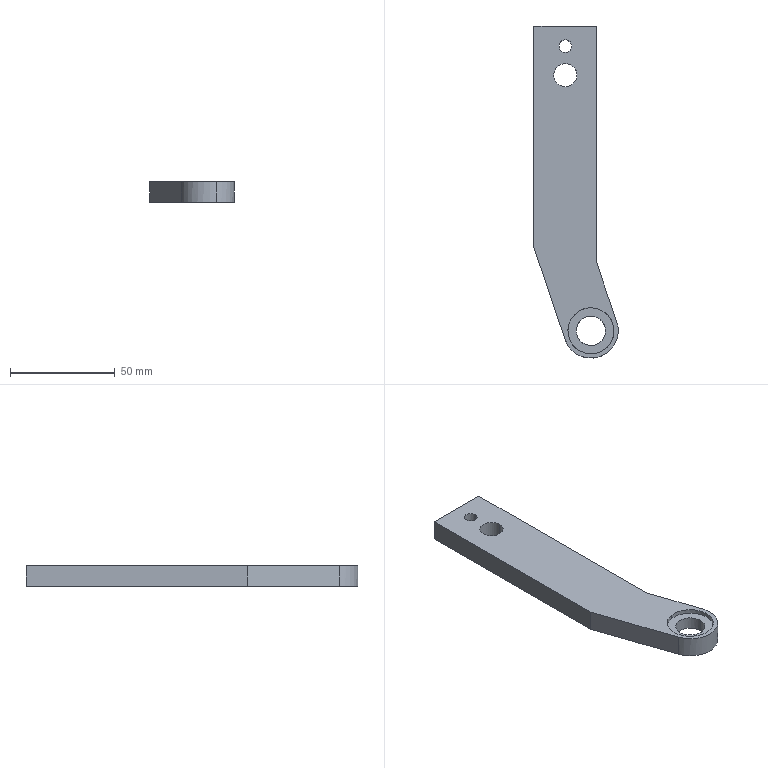Part | SolidWorks | features HoleWzd 2, BaseBody 1, Chamfer 1 | 1 solid | 23 faces | box 40.191 x 158.27 x 10 mm | volume 41618 mm3 | cylinder 12 | plane 9 | cone 2 | commonest cylinder face diameters 22 x4 6 x2 11 x2 14 x2 26 x2
STEP:
#1=CARTESIAN_POINT('',(409.071,348.177,19.477));
#2=VERTEX_POINT('',#1);
#3=CARTESIAN_POINT('',(403.071,348.177,19.477));
#4=VERTEX_POINT('',#3);
#5=CARTESIAN_POINT('',(406.071,348.177,19.477));
#6=DIRECTION('',(0.,0.,-1.));
#7=DIRECTION('',(-1.,0.,0.));
#8=AXIS2_PLACEMENT_3D('',#5,#6,#7);
#9=CIRCLE('',#8,3.);
#10=EDGE_CURVE('',#2,#4,#9,.T.);
#11=ORIENTED_EDGE('',*,*,#10,.F.);
#12=CARTESIAN_POINT('',(410.071,348.177,18.477));
#13=VERTEX_POINT('',#12);
#14=CARTESIAN_POINT('',(409.071,348.177,19.477));
#15=DIRECTION('',(0.7071,0.,-0.7071));
#16=VECTOR('',#15,1000.);
#17=LINE('',#14,#16);
#18=EDGE_CURVE('',#2,#13,#17,.T.);
#19=ORIENTED_EDGE('',*,*,#18,.T.);
#20=CARTESIAN_POINT('',(402.071,348.177,18.477));
#21=VERTEX_POINT('',#20);
#22=CARTESIAN_POINT('',(406.071,348.177,18.477));
#23=DIRECTION('',(0.,0.,1.));
#24=DIRECTION('',(-1.,0.,0.));
#25=AXIS2_PLACEMENT_3D('',#22,#23,#24);
#26=CIRCLE('',#25,4.);
#27=EDGE_CURVE('',#21,#13,#26,.T.);
#28=ORIENTED_EDGE('',*,*,#27,.F.);
#29=CARTESIAN_POINT('',(403.071,348.177,19.477));
#30=DIRECTION('',(-0.7071,0.,-0.7071));
#31=VECTOR('',#30,1000.);
#32=LINE('',#29,#31);
#33=EDGE_CURVE('',#4,#21,#32,.T.);
#34=ORIENTED_EDGE('',*,*,#33,.F.);
#35=EDGE_LOOP('',(#11,#19,#28,#34));
#36=FACE_OUTER_BOUND('',#35,.T.);
#37=CARTESIAN_POINT('',(406.071,348.177,19.477));
#38=DIRECTION('',(0.,0.,-1.));
#39=DIRECTION('',(-1.,0.,0.));
#40=AXIS2_PLACEMENT_3D('',#37,#38,#39);
#41=CONICAL_SURFACE('',#40,3.,0.7854);
#42=ADVANCED_FACE('',(#36),#41,.F.);
#43=CARTESIAN_POINT('',(411.563,334.317,18.477));
#44=VERTEX_POINT('',#43);
#45=CARTESIAN_POINT('',(400.563,334.317,18.477));
#46=VERTEX_POINT('',#45);
#47=CARTESIAN_POINT('',(411.563,334.317,18.477));
#48=CARTESIAN_POINT('',(411.563,323.317,18.477));
#49=CARTESIAN_POINT('',(400.563,323.317,18.477));
#50=CARTESIAN_POINT('',(400.563,334.317,18.477));
#51=(BOUNDED_CURVE()B_SPLINE_CURVE(3,(#47,#48,#49,#50),.UNSPECIFIED.,.F.,.F.)B_SPLINE_CURVE_WITH_KNOTS((4,4),(5.82,8.961),.UNSPECIFIED.)CURVE()GEOMETRIC_REPRESENTATION_ITEM()RATIONAL_B_SPLINE_CURVE((1.,0.3333,0.3333,1.))REPRESENTATION_ITEM(''));
#52=EDGE_CURVE('',#44,#46,#51,.T.);
#53=ORIENTED_EDGE('',*,*,#52,.T.);
#54=CARTESIAN_POINT('',(400.565,334.315,28.477));
#55=VERTEX_POINT('',#54);
#56=CARTESIAN_POINT('',(400.565,334.315,28.48));
#57=DIRECTION('',(0.0002857,-0.0001428,1.));
#58=VECTOR('',#57,1000.);
#59=LINE('',#56,#58);
#60=EDGE_CURVE('',#46,#55,#59,.T.);
#61=ORIENTED_EDGE('',*,*,#60,.T.);
#62=CARTESIAN_POINT('',(411.565,334.315,28.477));
#63=VERTEX_POINT('',#62);
#64=CARTESIAN_POINT('',(411.565,334.315,28.477));
#65=CARTESIAN_POINT('',(411.565,323.315,28.477));
#66=CARTESIAN_POINT('',(400.565,323.315,28.477));
#67=CARTESIAN_POINT('',(400.565,334.315,28.477));
#68=(BOUNDED_CURVE()B_SPLINE_CURVE(3,(#64,#65,#66,#67),.UNSPECIFIED.,.F.,.F.)B_SPLINE_CURVE_WITH_KNOTS((4,4),(5.82,8.961),.UNSPECIFIED.)CURVE()GEOMETRIC_REPRESENTATION_ITEM()RATIONAL_B_SPLINE_CURVE((1.,0.3333,0.3333,1.))REPRESENTATION_ITEM(''));
#69=EDGE_CURVE('',#63,#55,#68,.T.);
#70=ORIENTED_EDGE('',*,*,#69,.F.);
#71=CARTESIAN_POINT('',(411.565,334.315,28.477));
#72=DIRECTION('',(0.0002857,-0.0001428,1.));
#73=VECTOR('',#72,1000.);
#74=LINE('',#71,#73);
#75=EDGE_CURVE('',#44,#63,#74,.T.);
#76=ORIENTED_EDGE('',*,*,#75,.F.);
#77=EDGE_LOOP('',(#53,#61,#70,#76));
#78=FACE_OUTER_BOUND('',#77,.T.);
#79=CARTESIAN_POINT('',(406.065,334.315,28.478));
#80=DIRECTION('',(0.0002857,-0.0001428,1.));
#81=DIRECTION('',(1.,0.,-0.0002857));
#82=AXIS2_PLACEMENT_3D('',#79,#80,#81);
#83=CYLINDRICAL_SURFACE('',#82,5.5);
#84=ADVANCED_FACE('',(#78),#83,.F.);
#85=CARTESIAN_POINT('',(409.071,348.177,28.477));
#86=VERTEX_POINT('',#85);
#87=CARTESIAN_POINT('',(403.071,348.177,28.477));
#88=VERTEX_POINT('',#87);
#89=CARTESIAN_POINT('',(406.071,348.177,28.477));
#90=DIRECTION('',(0.,0.,-1.));
#91=DIRECTION('',(-1.,0.,0.));
#92=AXIS2_PLACEMENT_3D('',#89,#90,#91);
#93=CIRCLE('',#92,3.);
#94=EDGE_CURVE('',#86,#88,#93,.T.);
#95=ORIENTED_EDGE('',*,*,#94,.F.);
#96=CARTESIAN_POINT('',(409.071,348.177,18.477));
#97=DIRECTION('',(0.,0.,-1.));
#98=VECTOR('',#97,1000.);
#99=LINE('',#96,#98);
#100=EDGE_CURVE('',#86,#2,#99,.T.);
#101=ORIENTED_EDGE('',*,*,#100,.T.);
#102=ORIENTED_EDGE('',*,*,#10,.T.);
#103=CARTESIAN_POINT('',(403.071,348.177,18.477));
#104=DIRECTION('',(0.,0.,-1.));
#105=VECTOR('',#104,1000.);
#106=LINE('',#103,#105);
#107=EDGE_CURVE('',#88,#4,#106,.T.);
#108=ORIENTED_EDGE('',*,*,#107,.F.);
#109=EDGE_LOOP('',(#95,#101,#102,#108));
#110=FACE_OUTER_BOUND('',#109,.T.);
#111=CARTESIAN_POINT('',(406.071,348.177,18.477));
#112=DIRECTION('',(0.,0.,-1.));
#113=DIRECTION('',(-1.,0.,0.));
#114=AXIS2_PLACEMENT_3D('',#111,#112,#113);
#115=CYLINDRICAL_SURFACE('',#114,3.);
#116=ADVANCED_FACE('',(#110),#115,.F.);
#117=CARTESIAN_POINT('',(411.269,212.516,20.485));
#118=VERTEX_POINT('',#117);
#119=CARTESIAN_POINT('',(425.269,212.516,20.487));
#120=VERTEX_POINT('',#119);
#121=CARTESIAN_POINT('',(411.269,212.516,20.485));
#122=CARTESIAN_POINT('',(411.269,198.516,20.485));
#123=CARTESIAN_POINT('',(425.269,198.516,20.487));
#124=CARTESIAN_POINT('',(425.269,212.516,20.487));
#125=(BOUNDED_CURVE()B_SPLINE_CURVE(3,(#121,#122,#123,#124),.UNSPECIFIED.,.F.,.F.)B_SPLINE_CURVE_WITH_KNOTS((4,4),(3.138,6.28),.UNSPECIFIED.)CURVE()GEOMETRIC_REPRESENTATION_ITEM()RATIONAL_B_SPLINE_CURVE((1.,0.3333,0.3333,1.))REPRESENTATION_ITEM(''));
#126=EDGE_CURVE('',#118,#120,#125,.T.);
#127=ORIENTED_EDGE('',*,*,#126,.F.);
#128=CARTESIAN_POINT('',(411.269,212.516,26.469));
#129=VERTEX_POINT('',#128);
#130=CARTESIAN_POINT('',(411.269,212.516,18.477));
#131=DIRECTION('',(0.,0.,1.));
#132=VECTOR('',#131,1000.);
#133=LINE('',#130,#132);
#134=EDGE_CURVE('',#118,#129,#133,.T.);
#135=ORIENTED_EDGE('',*,*,#134,.T.);
#136=CARTESIAN_POINT('',(425.269,212.516,26.467));
#137=VERTEX_POINT('',#136);
#138=CARTESIAN_POINT('',(425.269,212.516,26.467));
#139=CARTESIAN_POINT('',(425.269,198.516,26.467));
#140=CARTESIAN_POINT('',(411.269,198.516,26.469));
#141=CARTESIAN_POINT('',(411.269,212.516,26.469));
#142=(BOUNDED_CURVE()B_SPLINE_CURVE(3,(#138,#139,#140,#141),.UNSPECIFIED.,.F.,.T.)B_SPLINE_CURVE_WITH_KNOTS((4,4),(3.145,6.287),.UNSPECIFIED.)CURVE()GEOMETRIC_REPRESENTATION_ITEM()RATIONAL_B_SPLINE_CURVE((1.,0.3333,0.3333,1.))REPRESENTATION_ITEM(''));
#143=EDGE_CURVE('',#137,#129,#142,.T.);
#144=ORIENTED_EDGE('',*,*,#143,.F.);
#145=CARTESIAN_POINT('',(425.269,212.516,18.477));
#146=DIRECTION('',(0.,0.,1.));
#147=VECTOR('',#146,1000.);
#148=LINE('',#145,#147);
#149=EDGE_CURVE('',#120,#137,#148,.T.);
#150=ORIENTED_EDGE('',*,*,#149,.F.);
#151=EDGE_LOOP('',(#127,#135,#144,#150));
#152=FACE_OUTER_BOUND('',#151,.T.);
#153=CARTESIAN_POINT('',(418.269,212.516,18.477));
#154=DIRECTION('',(0.,0.,1.));
#155=DIRECTION('',(1.,0.,0.));
#156=AXIS2_PLACEMENT_3D('',#153,#154,#155);
#157=CYLINDRICAL_SURFACE('',#156,7.);
#158=ADVANCED_FACE('',(#152),#157,.F.);
#159=CARTESIAN_POINT('',(416.566,223.384,18.477));
#160=VERTEX_POINT('',#159);
#161=CARTESIAN_POINT('',(419.971,201.649,18.477));
#162=VERTEX_POINT('',#161);
#163=CARTESIAN_POINT('',(416.566,223.384,18.477));
#164=CARTESIAN_POINT('',(394.831,219.979,18.477));
#165=CARTESIAN_POINT('',(398.236,198.244,18.477));
#166=CARTESIAN_POINT('',(419.971,201.649,18.477));
#167=(BOUNDED_CURVE()B_SPLINE_CURVE(3,(#163,#164,#165,#166),.UNSPECIFIED.,.F.,.F.)B_SPLINE_CURVE_WITH_KNOTS((4,4),(4.864,8.006),.UNSPECIFIED.)CURVE()GEOMETRIC_REPRESENTATION_ITEM()RATIONAL_B_SPLINE_CURVE((1.,0.3333,0.3333,1.))REPRESENTATION_ITEM(''));
#168=EDGE_CURVE('',#160,#162,#167,.T.);
#169=ORIENTED_EDGE('',*,*,#168,.F.);
#170=CARTESIAN_POINT('',(416.565,223.384,20.485));
#171=VERTEX_POINT('',#170);
#172=CARTESIAN_POINT('',(416.566,223.384,13.485));
#173=DIRECTION('',(-0.0001435,-0.000000521,1.));
#174=VECTOR('',#173,1000.);
#175=LINE('',#172,#174);
#176=EDGE_CURVE('',#160,#171,#175,.T.);
#177=ORIENTED_EDGE('',*,*,#176,.T.);
#178=CARTESIAN_POINT('',(419.97,201.649,20.486));
#179=VERTEX_POINT('',#178);
#180=CARTESIAN_POINT('',(418.268,212.516,20.486));
#181=DIRECTION('',(0.0001435,0.000000521,-1.));
#182=DIRECTION('',(-1.,0.,-0.0001435));
#183=AXIS2_PLACEMENT_3D('',#180,#181,#182);
#184=CIRCLE('',#183,11.);
#185=EDGE_CURVE('',#179,#171,#184,.T.);
#186=ORIENTED_EDGE('',*,*,#185,.F.);
#187=CARTESIAN_POINT('',(419.971,201.649,13.486));
#188=DIRECTION('',(-0.0001435,-0.000000521,1.));
#189=VECTOR('',#188,1000.);
#190=LINE('',#187,#189);
#191=EDGE_CURVE('',#162,#179,#190,.T.);
#192=ORIENTED_EDGE('',*,*,#191,.F.);
#193=EDGE_LOOP('',(#169,#177,#186,#192));
#194=FACE_OUTER_BOUND('',#193,.T.);
#195=CARTESIAN_POINT('',(418.269,212.516,13.486));
#196=DIRECTION('',(-0.0001435,-0.000000521,1.));
#197=DIRECTION('',(0.1548,-0.988,0.00002169));
#198=AXIS2_PLACEMENT_3D('',#195,#196,#197);
#199=CYLINDRICAL_SURFACE('',#198,11.);
#200=ADVANCED_FACE('',(#194),#199,.F.);
#201=CARTESIAN_POINT('',(416.566,223.384,28.477));
#202=VERTEX_POINT('',#201);
#203=CARTESIAN_POINT('',(419.971,201.649,28.477));
#204=VERTEX_POINT('',#203);
#205=CARTESIAN_POINT('',(416.566,223.384,28.477));
#206=CARTESIAN_POINT('',(438.301,226.789,28.477));
#207=CARTESIAN_POINT('',(441.706,205.054,28.477));
#208=CARTESIAN_POINT('',(419.971,201.649,28.477));
#209=(BOUNDED_CURVE()B_SPLINE_CURVE(3,(#205,#206,#207,#208),.UNSPECIFIED.,.F.,.T.)B_SPLINE_CURVE_WITH_KNOTS((4,4),(1.419,4.561),.UNSPECIFIED.)CURVE()GEOMETRIC_REPRESENTATION_ITEM()RATIONAL_B_SPLINE_CURVE((1.,0.3333,0.3333,1.))REPRESENTATION_ITEM(''));
#210=EDGE_CURVE('',#202,#204,#209,.T.);
#211=ORIENTED_EDGE('',*,*,#210,.F.);
#212=CARTESIAN_POINT('',(416.565,223.384,26.468));
#213=VERTEX_POINT('',#212);
#214=CARTESIAN_POINT('',(416.566,223.384,33.468));
#215=DIRECTION('',(-0.0001435,-0.000000521,-1.));
#216=VECTOR('',#215,1000.);
#217=LINE('',#214,#216);
#218=EDGE_CURVE('',#202,#213,#217,.T.);
#219=ORIENTED_EDGE('',*,*,#218,.T.);
#220=CARTESIAN_POINT('',(419.97,201.649,26.468));
#221=VERTEX_POINT('',#220);
#222=CARTESIAN_POINT('',(418.268,212.516,26.468));
#223=DIRECTION('',(0.0001435,0.000000521,1.));
#224=DIRECTION('',(0.1548,-0.988,-0.00002169));
#225=AXIS2_PLACEMENT_3D('',#222,#223,#224);
#226=CIRCLE('',#225,11.);
#227=EDGE_CURVE('',#221,#213,#226,.T.);
#228=ORIENTED_EDGE('',*,*,#227,.F.);
#229=CARTESIAN_POINT('',(419.971,201.649,33.468));
#230=DIRECTION('',(-0.0001435,-0.000000521,-1.));
#231=VECTOR('',#230,1000.);
#232=LINE('',#229,#231);
#233=EDGE_CURVE('',#204,#221,#232,.T.);
#234=ORIENTED_EDGE('',*,*,#233,.F.);
#235=EDGE_LOOP('',(#211,#219,#228,#234));
#236=FACE_OUTER_BOUND('',#235,.T.);
#237=CARTESIAN_POINT('',(418.269,212.516,33.468));
#238=DIRECTION('',(-0.0001435,-0.000000521,-1.));
#239=DIRECTION('',(0.1548,-0.988,-0.00002169));
#240=AXIS2_PLACEMENT_3D('',#237,#238,#239);
#241=CYLINDRICAL_SURFACE('',#240,11.);
#242=ADVANCED_FACE('',(#236),#241,.F.);
#243=CARTESIAN_POINT('',(422.618,200.265,18.477));
#244=VERTEX_POINT('',#243);
#245=CARTESIAN_POINT('',(405.95,208.362,18.477));
#246=VERTEX_POINT('',#245);
#247=CARTESIAN_POINT('',(422.618,200.265,18.477));
#248=CARTESIAN_POINT('',(415.351,197.686,18.477));
#249=CARTESIAN_POINT('',(408.414,201.055,18.477));
#250=CARTESIAN_POINT('',(405.95,208.362,18.477));
#251=(BOUNDED_CURVE()B_SPLINE_CURVE(3,(#247,#248,#249,#250),.UNSPECIFIED.,.F.,.F.)B_SPLINE_CURVE_WITH_KNOTS((4,4),(4.375,5.962),.UNSPECIFIED.)CURVE()GEOMETRIC_REPRESENTATION_ITEM()RATIONAL_B_SPLINE_CURVE((1.,0.801,0.801,1.))REPRESENTATION_ITEM(''));
#252=EDGE_CURVE('',#244,#246,#251,.T.);
#253=ORIENTED_EDGE('',*,*,#252,.F.);
#254=CARTESIAN_POINT('',(422.616,200.265,28.477));
#255=VERTEX_POINT('',#254);
#256=CARTESIAN_POINT('',(422.618,200.265,15.708));
#257=DIRECTION('',(-0.0001435,-0.000000521,1.));
#258=VECTOR('',#257,1000.);
#259=LINE('',#256,#258);
#260=EDGE_CURVE('',#244,#255,#259,.T.);
#261=ORIENTED_EDGE('',*,*,#260,.T.);
#262=CARTESIAN_POINT('',(405.949,208.362,28.477));
#263=VERTEX_POINT('',#262);
#264=CARTESIAN_POINT('',(405.949,208.362,28.477));
#265=CARTESIAN_POINT('',(408.413,201.055,28.477));
#266=CARTESIAN_POINT('',(415.349,197.686,28.477));
#267=CARTESIAN_POINT('',(422.616,200.265,28.477));
#268=(BOUNDED_CURVE()B_SPLINE_CURVE(3,(#264,#265,#266,#267),.UNSPECIFIED.,.F.,.F.)B_SPLINE_CURVE_WITH_KNOTS((4,4),(0.3216,1.908),.UNSPECIFIED.)CURVE()GEOMETRIC_REPRESENTATION_ITEM()RATIONAL_B_SPLINE_CURVE((1.,0.801,0.801,1.))REPRESENTATION_ITEM(''));
#269=EDGE_CURVE('',#263,#255,#268,.T.);
#270=ORIENTED_EDGE('',*,*,#269,.F.);
#271=CARTESIAN_POINT('',(405.949,208.362,28.477));
#272=DIRECTION('',(0.0001435,0.000000521,-1.));
#273=VECTOR('',#272,1000.);
#274=LINE('',#271,#273);
#275=EDGE_CURVE('',#263,#246,#274,.T.);
#276=ORIENTED_EDGE('',*,*,#275,.T.);
#277=EDGE_LOOP('',(#253,#261,#270,#276));
#278=FACE_OUTER_BOUND('',#277,.T.);
#279=CARTESIAN_POINT('',(418.269,212.516,15.707));
#280=DIRECTION('',(-0.0001435,-0.000000521,1.));
#281=DIRECTION('',(0.3345,-0.9424,0.00004751));
#282=AXIS2_PLACEMENT_3D('',#279,#280,#281);
#283=CYLINDRICAL_SURFACE('',#282,13.);
#284=ADVANCED_FACE('',(#278),#283,.T.);
#285=CARTESIAN_POINT('',(421.077,357.787,28.477));
#286=VERTEX_POINT('',#285);
#287=CARTESIAN_POINT('',(391.077,357.787,28.477));
#288=VERTEX_POINT('',#287);
#289=CARTESIAN_POINT('',(421.077,357.787,28.477));
#290=DIRECTION('',(-1.,-0.000000002,0.));
#291=VECTOR('',#290,1000.);
#292=LINE('',#289,#291);
#293=EDGE_CURVE('',#286,#288,#292,.T.);
#294=ORIENTED_EDGE('',*,*,#293,.F.);
#295=CARTESIAN_POINT('',(421.077,357.787,18.477));
#296=VERTEX_POINT('',#295);
#297=CARTESIAN_POINT('',(421.077,357.787,28.477));
#298=DIRECTION('',(0.,0.,-1.));
#299=VECTOR('',#298,1000.);
#300=LINE('',#297,#299);
#301=EDGE_CURVE('',#286,#296,#300,.T.);
#302=ORIENTED_EDGE('',*,*,#301,.T.);
#303=CARTESIAN_POINT('',(391.077,357.787,18.477));
#304=VERTEX_POINT('',#303);
#305=CARTESIAN_POINT('',(391.077,357.787,18.477));
#306=DIRECTION('',(1.,0.000000002,0.));
#307=VECTOR('',#306,1000.);
#308=LINE('',#305,#307);
#309=EDGE_CURVE('',#304,#296,#308,.T.);
#310=ORIENTED_EDGE('',*,*,#309,.F.);
#311=CARTESIAN_POINT('',(391.077,357.787,28.477));
#312=DIRECTION('',(0.,0.,-1.));
#313=VECTOR('',#312,1000.);
#314=LINE('',#311,#313);
#315=EDGE_CURVE('',#288,#304,#314,.T.);
#316=ORIENTED_EDGE('',*,*,#315,.F.);
#317=EDGE_LOOP('',(#294,#302,#310,#316));
#318=FACE_OUTER_BOUND('',#317,.T.);
#319=CARTESIAN_POINT('',(405.902,357.787,18.477));
#320=DIRECTION('',(0.,1.,0.));
#321=DIRECTION('',(1.,0.,0.));
#322=AXIS2_PLACEMENT_3D('',#319,#320,#321);
#323=PLANE('',#322);
#324=ADVANCED_FACE('',(#318),#323,.T.);
#325=CARTESIAN_POINT('',(421.077,244.864,28.477));
#326=VERTEX_POINT('',#325);
#327=CARTESIAN_POINT('',(421.077,244.864,28.477));
#328=DIRECTION('',(-0.000000041,1.,0.));
#329=VECTOR('',#328,1000.);
#330=LINE('',#327,#329);
#331=EDGE_CURVE('',#326,#286,#330,.T.);
#332=ORIENTED_EDGE('',*,*,#331,.F.);
#333=CARTESIAN_POINT('',(421.077,244.868,18.477));
#334=VERTEX_POINT('',#333);
#335=CARTESIAN_POINT('',(421.077,244.868,18.477));
#336=DIRECTION('',(0.,-0.000426,1.));
#337=VECTOR('',#336,1000.);
#338=LINE('',#335,#337);
#339=EDGE_CURVE('',#334,#326,#338,.T.);
#340=ORIENTED_EDGE('',*,*,#339,.F.);
#341=CARTESIAN_POINT('',(421.077,357.787,18.477));
#342=DIRECTION('',(0.000000041,-1.,0.));
#343=VECTOR('',#342,1000.);
#344=LINE('',#341,#343);
#345=EDGE_CURVE('',#296,#334,#344,.T.);
#346=ORIENTED_EDGE('',*,*,#345,.F.);
#347=ORIENTED_EDGE('',*,*,#301,.F.);
#348=EDGE_LOOP('',(#332,#340,#346,#347));
#349=FACE_OUTER_BOUND('',#348,.T.);
#350=CARTESIAN_POINT('',(421.077,334.785,18.477));
#351=DIRECTION('',(1.,0.000000041,0.));
#352=DIRECTION('',(0.,-0.0001428,-1.));
#353=AXIS2_PLACEMENT_3D('',#350,#351,#352);
#354=PLANE('',#353);
#355=ADVANCED_FACE('',(#349),#354,.T.);
#356=CARTESIAN_POINT('',(430.585,216.671,28.477));
#357=VERTEX_POINT('',#356);
#358=CARTESIAN_POINT('',(430.585,216.671,28.477));
#359=DIRECTION('',(-0.3196,0.9476,0.));
#360=VECTOR('',#359,1000.);
#361=LINE('',#358,#360);
#362=EDGE_CURVE('',#357,#326,#361,.T.);
#363=ORIENTED_EDGE('',*,*,#362,.F.);
#364=CARTESIAN_POINT('',(430.587,216.671,18.477));
#365=VERTEX_POINT('',#364);
#366=CARTESIAN_POINT('',(430.587,216.671,18.477));
#367=DIRECTION('',(-0.0001435,-0.000000521,1.));
#368=VECTOR('',#367,1000.);
#369=LINE('',#366,#368);
#370=EDGE_CURVE('',#365,#357,#369,.T.);
#371=ORIENTED_EDGE('',*,*,#370,.F.);
#372=CARTESIAN_POINT('',(421.077,244.868,18.477));
#373=DIRECTION('',(0.3196,-0.9476,0.));
#374=VECTOR('',#373,1000.);
#375=LINE('',#372,#374);
#376=EDGE_CURVE('',#334,#365,#375,.T.);
#377=ORIENTED_EDGE('',*,*,#376,.F.);
#378=ORIENTED_EDGE('',*,*,#339,.T.);
#379=EDGE_LOOP('',(#363,#371,#377,#378));
#380=FACE_OUTER_BOUND('',#379,.T.);
#381=CARTESIAN_POINT('',(406.851,287.053,16.039));
#382=DIRECTION('',(0.9476,0.3196,0.0001361));
#383=DIRECTION('',(0.,0.000426,-1.));
#384=AXIS2_PLACEMENT_3D('',#381,#382,#383);
#385=PLANE('',#384);
#386=ADVANCED_FACE('',(#380),#385,.T.);
#387=ORIENTED_EDGE('',*,*,#260,.F.);
#388=CARTESIAN_POINT('',(430.587,216.671,18.477));
#389=CARTESIAN_POINT('',(432.99,209.545,18.477));
#390=CARTESIAN_POINT('',(429.704,202.781,18.477));
#391=CARTESIAN_POINT('',(422.618,200.265,18.477));
#392=(BOUNDED_CURVE()B_SPLINE_CURVE(3,(#388,#389,#390,#391),.UNSPECIFIED.,.F.,.F.)B_SPLINE_CURVE_WITH_KNOTS((4,4),(2.82,4.375),.UNSPECIFIED.)CURVE()GEOMETRIC_REPRESENTATION_ITEM()RATIONAL_B_SPLINE_CURVE((1.,0.8085,0.8085,1.))REPRESENTATION_ITEM(''));
#393=EDGE_CURVE('',#365,#244,#392,.T.);
#394=ORIENTED_EDGE('',*,*,#393,.F.);
#395=ORIENTED_EDGE('',*,*,#370,.T.);
#396=CARTESIAN_POINT('',(422.616,200.265,28.477));
#397=CARTESIAN_POINT('',(429.703,202.781,28.477));
#398=CARTESIAN_POINT('',(432.988,209.545,28.477));
#399=CARTESIAN_POINT('',(430.585,216.671,28.477));
#400=(BOUNDED_CURVE()B_SPLINE_CURVE(3,(#396,#397,#398,#399),.UNSPECIFIED.,.F.,.F.)B_SPLINE_CURVE_WITH_KNOTS((4,4),(1.908,3.463),.UNSPECIFIED.)CURVE()GEOMETRIC_REPRESENTATION_ITEM()RATIONAL_B_SPLINE_CURVE((1.,0.8085,0.8085,1.))REPRESENTATION_ITEM(''));
#401=EDGE_CURVE('',#255,#357,#400,.T.);
#402=ORIENTED_EDGE('',*,*,#401,.F.);
#403=EDGE_LOOP('',(#387,#394,#395,#402));
#404=FACE_OUTER_BOUND('',#403,.T.);
#405=CARTESIAN_POINT('',(418.269,212.516,15.707));
#406=DIRECTION('',(-0.0001435,-0.000000521,1.));
#407=DIRECTION('',(0.3345,-0.9424,0.00004751));
#408=AXIS2_PLACEMENT_3D('',#405,#406,#407);
#409=CYLINDRICAL_SURFACE('',#408,13.);
#410=ADVANCED_FACE('',(#404),#409,.T.);
#411=CARTESIAN_POINT('',(391.077,252.458,28.477));
#412=VERTEX_POINT('',#411);
#413=CARTESIAN_POINT('',(391.077,252.463,18.477));
#414=VERTEX_POINT('',#413);
#415=CARTESIAN_POINT('',(391.077,252.458,28.477));
#416=DIRECTION('',(0.,0.000426,-1.));
#417=VECTOR('',#416,1000.);
#418=LINE('',#415,#417);
#419=EDGE_CURVE('',#412,#414,#418,.T.);
#420=ORIENTED_EDGE('',*,*,#419,.T.);
#421=CARTESIAN_POINT('',(405.95,208.362,18.477));
#422=DIRECTION('',(-0.3196,0.9476,0.));
#423=VECTOR('',#422,1000.);
#424=LINE('',#421,#423);
#425=EDGE_CURVE('',#246,#414,#424,.T.);
#426=ORIENTED_EDGE('',*,*,#425,.F.);
#427=ORIENTED_EDGE('',*,*,#275,.F.);
#428=CARTESIAN_POINT('',(391.077,252.458,28.477));
#429=DIRECTION('',(0.3196,-0.9476,0.));
#430=VECTOR('',#429,1000.);
#431=LINE('',#428,#430);
#432=EDGE_CURVE('',#412,#263,#431,.T.);
#433=ORIENTED_EDGE('',*,*,#432,.F.);
#434=EDGE_LOOP('',(#420,#426,#427,#433));
#435=FACE_OUTER_BOUND('',#434,.T.);
#436=CARTESIAN_POINT('',(382.346,278.354,16.047));
#437=DIRECTION('',(-0.9476,-0.3196,-0.0001361));
#438=DIRECTION('',(-0.3196,0.9476,0.));
#439=AXIS2_PLACEMENT_3D('',#436,#437,#438);
#440=PLANE('',#439);
#441=ADVANCED_FACE('',(#435),#440,.T.);
#442=ORIENTED_EDGE('',*,*,#27,.T.);
#443=CARTESIAN_POINT('',(406.071,348.177,18.477));
#444=DIRECTION('',(0.,0.,1.));
#445=DIRECTION('',(-1.,0.,0.));
#446=AXIS2_PLACEMENT_3D('',#443,#444,#445);
#447=CIRCLE('',#446,4.);
#448=EDGE_CURVE('',#13,#21,#447,.T.);
#449=ORIENTED_EDGE('',*,*,#448,.T.);
#450=EDGE_LOOP('',(#442,#449));
#451=FACE_BOUND('',#450,.T.);
#452=ORIENTED_EDGE('',*,*,#52,.F.);
#453=CARTESIAN_POINT('',(400.563,334.317,18.477));
#454=CARTESIAN_POINT('',(400.563,345.317,18.477));
#455=CARTESIAN_POINT('',(411.563,345.317,18.477));
#456=CARTESIAN_POINT('',(411.563,334.317,18.477));
#457=(BOUNDED_CURVE()B_SPLINE_CURVE(3,(#453,#454,#455,#456),.UNSPECIFIED.,.F.,.F.)B_SPLINE_CURVE_WITH_KNOTS((4,4),(2.678,5.82),.UNSPECIFIED.)CURVE()GEOMETRIC_REPRESENTATION_ITEM()RATIONAL_B_SPLINE_CURVE((1.,0.3333,0.3333,1.))REPRESENTATION_ITEM(''));
#458=EDGE_CURVE('',#46,#44,#457,.T.);
#459=ORIENTED_EDGE('',*,*,#458,.F.);
#460=EDGE_LOOP('',(#452,#459));
#461=FACE_BOUND('',#460,.T.);
#462=CARTESIAN_POINT('',(419.971,201.649,18.477));
#463=CARTESIAN_POINT('',(441.706,205.054,18.477));
#464=CARTESIAN_POINT('',(438.301,226.789,18.477));
#465=CARTESIAN_POINT('',(416.566,223.384,18.477));
#466=(BOUNDED_CURVE()B_SPLINE_CURVE(3,(#462,#463,#464,#465),.UNSPECIFIED.,.F.,.F.)B_SPLINE_CURVE_WITH_KNOTS((4,4),(1.723,4.864),.UNSPECIFIED.)CURVE()GEOMETRIC_REPRESENTATION_ITEM()RATIONAL_B_SPLINE_CURVE((1.,0.3333,0.3333,1.))REPRESENTATION_ITEM(''));
#467=EDGE_CURVE('',#162,#160,#466,.T.);
#468=ORIENTED_EDGE('',*,*,#467,.T.);
#469=ORIENTED_EDGE('',*,*,#168,.T.);
#470=EDGE_LOOP('',(#468,#469));
#471=FACE_BOUND('',#470,.T.);
#472=CARTESIAN_POINT('',(391.077,252.463,18.477));
#473=DIRECTION('',(-0.000000041,1.,0.));
#474=VECTOR('',#473,1000.);
#475=LINE('',#472,#474);
#476=EDGE_CURVE('',#414,#304,#475,.T.);
#477=ORIENTED_EDGE('',*,*,#476,.T.);
#478=ORIENTED_EDGE('',*,*,#309,.T.);
#479=ORIENTED_EDGE('',*,*,#345,.T.);
#480=ORIENTED_EDGE('',*,*,#376,.T.);
#481=ORIENTED_EDGE('',*,*,#393,.T.);
#482=ORIENTED_EDGE('',*,*,#252,.T.);
#483=ORIENTED_EDGE('',*,*,#425,.T.);
#484=EDGE_LOOP('',(#477,#478,#479,#480,#481,#482,#483));
#485=FACE_OUTER_BOUND('',#484,.T.);
#486=CARTESIAN_POINT('',(393.902,284.761,18.477));
#487=DIRECTION('',(0.,0.,-1.));
#488=DIRECTION('',(0.,-1.,0.));
#489=AXIS2_PLACEMENT_3D('',#486,#487,#488);
#490=PLANE('',#489);
#491=ADVANCED_FACE('',(#451,#461,#471,#485),#490,.T.);
#492=ORIENTED_EDGE('',*,*,#69,.T.);
#493=CARTESIAN_POINT('',(400.565,334.315,28.477));
#494=CARTESIAN_POINT('',(400.565,345.315,28.477));
#495=CARTESIAN_POINT('',(411.565,345.315,28.477));
#496=CARTESIAN_POINT('',(411.565,334.315,28.477));
#497=(BOUNDED_CURVE()B_SPLINE_CURVE(3,(#493,#494,#495,#496),.UNSPECIFIED.,.F.,.F.)B_SPLINE_CURVE_WITH_KNOTS((4,4),(2.678,5.82),.UNSPECIFIED.)CURVE()GEOMETRIC_REPRESENTATION_ITEM()RATIONAL_B_SPLINE_CURVE((1.,0.3333,0.3333,1.))REPRESENTATION_ITEM(''));
#498=EDGE_CURVE('',#55,#63,#497,.T.);
#499=ORIENTED_EDGE('',*,*,#498,.T.);
#500=EDGE_LOOP('',(#492,#499));
#501=FACE_BOUND('',#500,.T.);
#502=CARTESIAN_POINT('',(406.071,348.177,28.477));
#503=DIRECTION('',(0.,0.,-1.));
#504=DIRECTION('',(-1.,0.,0.));
#505=AXIS2_PLACEMENT_3D('',#502,#503,#504);
#506=CIRCLE('',#505,3.);
#507=EDGE_CURVE('',#88,#86,#506,.T.);
#508=ORIENTED_EDGE('',*,*,#507,.T.);
#509=ORIENTED_EDGE('',*,*,#94,.T.);
#510=EDGE_LOOP('',(#508,#509));
#511=FACE_BOUND('',#510,.T.);
#512=CARTESIAN_POINT('',(419.971,201.649,28.477));
#513=CARTESIAN_POINT('',(398.236,198.244,28.477));
#514=CARTESIAN_POINT('',(394.831,219.979,28.477));
#515=CARTESIAN_POINT('',(416.566,223.384,28.477));
#516=(BOUNDED_CURVE()B_SPLINE_CURVE(3,(#512,#513,#514,#515),.UNSPECIFIED.,.F.,.T.)B_SPLINE_CURVE_WITH_KNOTS((4,4),(4.561,7.702),.UNSPECIFIED.)CURVE()GEOMETRIC_REPRESENTATION_ITEM()RATIONAL_B_SPLINE_CURVE((1.,0.3333,0.3333,1.))REPRESENTATION_ITEM(''));
#517=EDGE_CURVE('',#204,#202,#516,.T.);
#518=ORIENTED_EDGE('',*,*,#517,.T.);
#519=ORIENTED_EDGE('',*,*,#210,.T.);
#520=EDGE_LOOP('',(#518,#519));
#521=FACE_BOUND('',#520,.T.);
#522=ORIENTED_EDGE('',*,*,#432,.T.);
#523=ORIENTED_EDGE('',*,*,#269,.T.);
#524=ORIENTED_EDGE('',*,*,#401,.T.);
#525=ORIENTED_EDGE('',*,*,#362,.T.);
#526=ORIENTED_EDGE('',*,*,#331,.T.);
#527=ORIENTED_EDGE('',*,*,#293,.T.);
#528=CARTESIAN_POINT('',(391.077,357.787,28.477));
#529=DIRECTION('',(0.000000041,-1.,0.));
#530=VECTOR('',#529,1000.);
#531=LINE('',#528,#530);
#532=EDGE_CURVE('',#288,#412,#531,.T.);
#533=ORIENTED_EDGE('',*,*,#532,.T.);
#534=EDGE_LOOP('',(#522,#523,#524,#525,#526,#527,#533));
#535=FACE_OUTER_BOUND('',#534,.T.);
#536=CARTESIAN_POINT('',(393.902,284.761,28.477));
#537=DIRECTION('',(0.,0.,-1.));
#538=DIRECTION('',(0.,-1.,0.));
#539=AXIS2_PLACEMENT_3D('',#536,#537,#538);
#540=PLANE('',#539);
#541=ADVANCED_FACE('',(#501,#511,#521,#535),#540,.F.);
#542=ORIENTED_EDGE('',*,*,#315,.T.);
#543=ORIENTED_EDGE('',*,*,#476,.F.);
#544=ORIENTED_EDGE('',*,*,#419,.F.);
#545=ORIENTED_EDGE('',*,*,#532,.F.);
#546=EDGE_LOOP('',(#542,#543,#544,#545));
#547=FACE_OUTER_BOUND('',#546,.T.);
#548=CARTESIAN_POINT('',(391.077,334.785,18.477));
#549=DIRECTION('',(-1.,-0.000000041,0.));
#550=DIRECTION('',(-0.000000041,1.,0.));
#551=AXIS2_PLACEMENT_3D('',#548,#549,#550);
#552=PLANE('',#551);
#553=ADVANCED_FACE('',(#547),#552,.T.);
#554=ORIENTED_EDGE('',*,*,#218,.F.);
#555=ORIENTED_EDGE('',*,*,#517,.F.);
#556=ORIENTED_EDGE('',*,*,#233,.T.);
#557=CARTESIAN_POINT('',(418.268,212.516,26.468));
#558=DIRECTION('',(0.0001435,0.000000521,1.));
#559=DIRECTION('',(0.1548,-0.988,-0.00002169));
#560=AXIS2_PLACEMENT_3D('',#557,#558,#559);
#561=CIRCLE('',#560,11.);
#562=EDGE_CURVE('',#213,#221,#561,.T.);
#563=ORIENTED_EDGE('',*,*,#562,.F.);
#564=EDGE_LOOP('',(#554,#555,#556,#563));
#565=FACE_OUTER_BOUND('',#564,.T.);
#566=CARTESIAN_POINT('',(418.269,212.516,33.468));
#567=DIRECTION('',(-0.0001435,-0.000000521,-1.));
#568=DIRECTION('',(0.1548,-0.988,-0.00002169));
#569=AXIS2_PLACEMENT_3D('',#566,#567,#568);
#570=CYLINDRICAL_SURFACE('',#569,11.);
#571=ADVANCED_FACE('',(#565),#570,.F.);
#572=ORIENTED_EDGE('',*,*,#143,.T.);
#573=CARTESIAN_POINT('',(411.269,212.516,26.469));
#574=CARTESIAN_POINT('',(411.269,226.516,26.469));
#575=CARTESIAN_POINT('',(425.269,226.516,26.467));
#576=CARTESIAN_POINT('',(425.269,212.516,26.467));
#577=(BOUNDED_CURVE()B_SPLINE_CURVE(3,(#573,#574,#575,#576),.UNSPECIFIED.,.F.,.F.)B_SPLINE_CURVE_WITH_KNOTS((4,4),(0.003633,3.145),.UNSPECIFIED.)CURVE()GEOMETRIC_REPRESENTATION_ITEM()RATIONAL_B_SPLINE_CURVE((1.,0.3333,0.3333,1.))REPRESENTATION_ITEM(''));
#578=EDGE_CURVE('',#129,#137,#577,.T.);
#579=ORIENTED_EDGE('',*,*,#578,.T.);
#580=EDGE_LOOP('',(#572,#579));
#581=FACE_BOUND('',#580,.T.);
#582=ORIENTED_EDGE('',*,*,#227,.T.);
#583=ORIENTED_EDGE('',*,*,#562,.T.);
#584=EDGE_LOOP('',(#582,#583));
#585=FACE_OUTER_BOUND('',#584,.T.);
#586=CARTESIAN_POINT('',(418.268,212.516,26.468));
#587=DIRECTION('',(-0.0001435,-0.000000521,-1.));
#588=DIRECTION('',(-1.,0.,0.0001435));
#589=AXIS2_PLACEMENT_3D('',#586,#587,#588);
#590=PLANE('',#589);
#591=ADVANCED_FACE('',(#581,#585),#590,.F.);
#592=ORIENTED_EDGE('',*,*,#176,.F.);
#593=ORIENTED_EDGE('',*,*,#467,.F.);
#594=ORIENTED_EDGE('',*,*,#191,.T.);
#595=CARTESIAN_POINT('',(418.268,212.516,20.486));
#596=DIRECTION('',(0.0001435,0.000000521,-1.));
#597=DIRECTION('',(-1.,0.,-0.0001435));
#598=AXIS2_PLACEMENT_3D('',#595,#596,#597);
#599=CIRCLE('',#598,11.);
#600=EDGE_CURVE('',#171,#179,#599,.T.);
#601=ORIENTED_EDGE('',*,*,#600,.F.);
#602=EDGE_LOOP('',(#592,#593,#594,#601));
#603=FACE_OUTER_BOUND('',#602,.T.);
#604=CARTESIAN_POINT('',(418.269,212.516,13.486));
#605=DIRECTION('',(-0.0001435,-0.000000521,1.));
#606=DIRECTION('',(0.1548,-0.988,0.00002169));
#607=AXIS2_PLACEMENT_3D('',#604,#605,#606);
#608=CYLINDRICAL_SURFACE('',#607,11.);
#609=ADVANCED_FACE('',(#603),#608,.F.);
#610=CARTESIAN_POINT('',(425.268,212.542,20.487));
#611=VERTEX_POINT('',#610);
#612=CARTESIAN_POINT('',(418.269,212.516,20.487));
#613=DIRECTION('',(0.,0.,1.));
#614=DIRECTION('',(1.,0.,0.));
#615=AXIS2_PLACEMENT_3D('',#612,#613,#614);
#616=CIRCLE('',#615,7.);
#617=EDGE_CURVE('',#120,#611,#616,.T.);
#618=ORIENTED_EDGE('',*,*,#617,.T.);
#619=CARTESIAN_POINT('',(425.268,212.542,20.487));
#620=CARTESIAN_POINT('',(425.218,226.491,20.487));
#621=CARTESIAN_POINT('',(411.269,226.466,20.485));
#622=CARTESIAN_POINT('',(411.269,212.516,20.485));
#623=(BOUNDED_CURVE()B_SPLINE_CURVE(3,(#619,#620,#621,#622),.UNSPECIFIED.,.F.,.F.)B_SPLINE_CURVE_WITH_KNOTS((4,4),(0.,3.138),.UNSPECIFIED.)CURVE()GEOMETRIC_REPRESENTATION_ITEM()RATIONAL_B_SPLINE_CURVE((1.,0.3345,0.3345,1.))REPRESENTATION_ITEM(''));
#624=EDGE_CURVE('',#611,#118,#623,.T.);
#625=ORIENTED_EDGE('',*,*,#624,.T.);
#626=ORIENTED_EDGE('',*,*,#126,.T.);
#627=EDGE_LOOP('',(#618,#625,#626));
#628=FACE_BOUND('',#627,.T.);
#629=ORIENTED_EDGE('',*,*,#185,.T.);
#630=ORIENTED_EDGE('',*,*,#600,.T.);
#631=EDGE_LOOP('',(#629,#630));
#632=FACE_OUTER_BOUND('',#631,.T.);
#633=CARTESIAN_POINT('',(418.268,212.516,20.486));
#634=DIRECTION('',(-0.0001435,-0.000000521,1.));
#635=DIRECTION('',(-0.003633,1.,0.));
#636=AXIS2_PLACEMENT_3D('',#633,#634,#635);
#637=PLANE('',#636);
#638=ADVANCED_FACE('',(#628,#632),#637,.F.);
#639=ORIENTED_EDGE('',*,*,#134,.F.);
#640=ORIENTED_EDGE('',*,*,#624,.F.);
#641=ORIENTED_EDGE('',*,*,#617,.F.);
#642=ORIENTED_EDGE('',*,*,#149,.T.);
#643=ORIENTED_EDGE('',*,*,#578,.F.);
#644=EDGE_LOOP('',(#639,#640,#641,#642,#643));
#645=FACE_OUTER_BOUND('',#644,.T.);
#646=CARTESIAN_POINT('',(418.269,212.516,18.477));
#647=DIRECTION('',(0.,0.,1.));
#648=DIRECTION('',(1.,0.,0.));
#649=AXIS2_PLACEMENT_3D('',#646,#647,#648);
#650=CYLINDRICAL_SURFACE('',#649,7.);
#651=ADVANCED_FACE('',(#645),#650,.F.);
#652=ORIENTED_EDGE('',*,*,#100,.F.);
#653=ORIENTED_EDGE('',*,*,#507,.F.);
#654=ORIENTED_EDGE('',*,*,#107,.T.);
#655=CARTESIAN_POINT('',(406.071,348.177,19.477));
#656=DIRECTION('',(0.,0.,-1.));
#657=DIRECTION('',(-1.,0.,0.));
#658=AXIS2_PLACEMENT_3D('',#655,#656,#657);
#659=CIRCLE('',#658,3.);
#660=EDGE_CURVE('',#4,#2,#659,.T.);
#661=ORIENTED_EDGE('',*,*,#660,.T.);
#662=EDGE_LOOP('',(#652,#653,#654,#661));
#663=FACE_OUTER_BOUND('',#662,.T.);
#664=CARTESIAN_POINT('',(406.071,348.177,18.477));
#665=DIRECTION('',(0.,0.,-1.));
#666=DIRECTION('',(-1.,0.,0.));
#667=AXIS2_PLACEMENT_3D('',#664,#665,#666);
#668=CYLINDRICAL_SURFACE('',#667,3.);
#669=ADVANCED_FACE('',(#663),#668,.F.);
#670=ORIENTED_EDGE('',*,*,#60,.F.);
#671=ORIENTED_EDGE('',*,*,#458,.T.);
#672=ORIENTED_EDGE('',*,*,#75,.T.);
#673=ORIENTED_EDGE('',*,*,#498,.F.);
#674=EDGE_LOOP('',(#670,#671,#672,#673));
#675=FACE_OUTER_BOUND('',#674,.T.);
#676=CARTESIAN_POINT('',(406.065,334.315,28.478));
#677=DIRECTION('',(0.0002857,-0.0001428,1.));
#678=DIRECTION('',(1.,0.,-0.0002857));
#679=AXIS2_PLACEMENT_3D('',#676,#677,#678);
#680=CYLINDRICAL_SURFACE('',#679,5.5);
#681=ADVANCED_FACE('',(#675),#680,.F.);
#682=ORIENTED_EDGE('',*,*,#18,.F.);
#683=ORIENTED_EDGE('',*,*,#660,.F.);
#684=ORIENTED_EDGE('',*,*,#33,.T.);
#685=ORIENTED_EDGE('',*,*,#448,.F.);
#686=EDGE_LOOP('',(#682,#683,#684,#685));
#687=FACE_OUTER_BOUND('',#686,.T.);
#688=CARTESIAN_POINT('',(406.071,348.177,19.477));
#689=DIRECTION('',(0.,0.,-1.));
#690=DIRECTION('',(-1.,0.,0.));
#691=AXIS2_PLACEMENT_3D('',#688,#689,#690);
#692=CONICAL_SURFACE('',#691,3.,0.7854);
#693=ADVANCED_FACE('',(#687),#692,.F.);
#694=CLOSED_SHELL('',(#42,#84,#116,#158,#200,#242,#284,#324,#355,#386,#410,#441,#491,#541,#553,#571,#591,#609,#638,#651,#669,#681,#693));
#695=MANIFOLD_SOLID_BREP('',#694);
#696=CARTESIAN_POINT('',(0.,0.,0.));
#697=DIRECTION('',(0.,0.,1.));
#698=DIRECTION('',(1.,0.,0.));
#699=AXIS2_PLACEMENT_3D('',#696,#697,#698);
#700=(LENGTH_UNIT()NAMED_UNIT(*)SI_UNIT(.MILLI.,.METRE.));
#701=UNCERTAINTY_MEASURE_WITH_UNIT(LENGTH_MEASURE(0.00001),#700,'','');
#702=(NAMED_UNIT(*)PLANE_ANGLE_UNIT()SI_UNIT($,.RADIAN.));
#703=(NAMED_UNIT(*)SI_UNIT($,.STERADIAN.)SOLID_ANGLE_UNIT());
#704=(GEOMETRIC_REPRESENTATION_CONTEXT(3)GLOBAL_UNCERTAINTY_ASSIGNED_CONTEXT((#701))GLOBAL_UNIT_ASSIGNED_CONTEXT((#700,#702,#703))REPRESENTATION_CONTEXT('',''));
#705=ADVANCED_BREP_SHAPE_REPRESENTATION('',(#695,#699),#704);